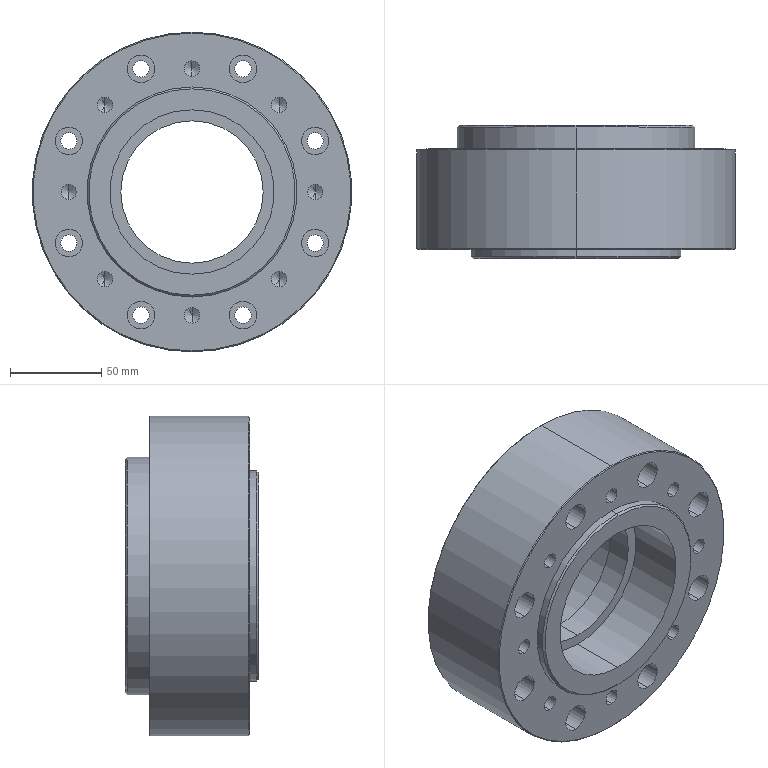Part | SolidWorks | features ICE 6, CirPattern 3, HoleWzd 3, Chamfer 2, Extrusion 1 | 1 solid | 122 faces | box 175 x 73 x 175 mm | volume 1030889 mm3 | cylinder 72 | cone 36 | plane 14 | commonest cylinder face diameters 8.5 x16 9 x16 15 x16 4.2 x12 90 x4 78 x2